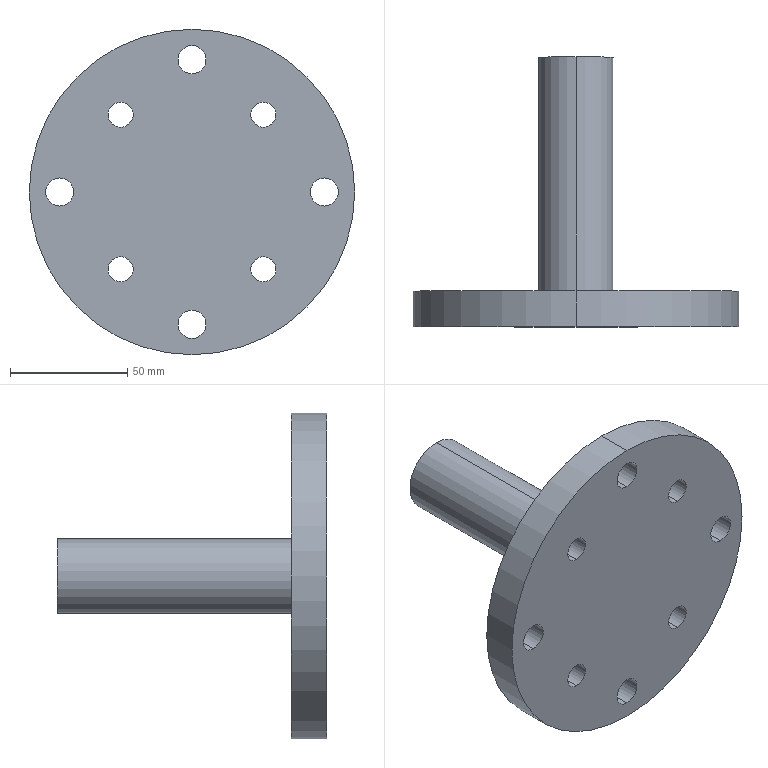Part | SolidWorks | features ICE 4, Cut 1, Extrusion 1, Scale 1 | 1 solid | 26 faces | box 139 x 115.24 x 139 mm | volume 246251 mm3 | cylinder 22 | plane 4 | commonest cylinder face diameters 10.668 x8 12 x8 26 x2 32 x2 139 x2
STEP:
#1=CARTESIAN_POINT('',(0.,0.,-69.5));
#2=VERTEX_POINT('',#1);
#3=CARTESIAN_POINT('',(0.,0.,69.5));
#4=VERTEX_POINT('',#3);
#5=CARTESIAN_POINT('',(0.,0.,0.));
#6=DIRECTION('',(0.,-1.,0.));
#7=DIRECTION('',(0.,0.,1.));
#8=AXIS2_PLACEMENT_3D('',#5,#6,#7);
#9=CIRCLE('',#8,69.5);
#10=EDGE_CURVE('',#2,#4,#9,.T.);
#11=ORIENTED_EDGE('',*,*,#10,.T.);
#12=CARTESIAN_POINT('',(0.,-15.24,69.5));
#13=VERTEX_POINT('',#12);
#14=CARTESIAN_POINT('',(0.,196.576,69.5));
#15=DIRECTION('',(0.,-1.,0.));
#16=VECTOR('',#15,1000.);
#17=LINE('',#14,#16);
#18=EDGE_CURVE('',#4,#13,#17,.T.);
#19=ORIENTED_EDGE('',*,*,#18,.T.);
#20=CARTESIAN_POINT('',(0.,-15.24,-69.5));
#21=VERTEX_POINT('',#20);
#22=CARTESIAN_POINT('',(0.,-15.24,0.));
#23=DIRECTION('',(0.,-1.,0.));
#24=DIRECTION('',(0.,0.,-1.));
#25=AXIS2_PLACEMENT_3D('',#22,#23,#24);
#26=CIRCLE('',#25,69.5);
#27=EDGE_CURVE('',#21,#13,#26,.T.);
#28=ORIENTED_EDGE('',*,*,#27,.F.);
#29=CARTESIAN_POINT('',(0.,196.576,-69.5));
#30=DIRECTION('',(0.,-1.,0.));
#31=VECTOR('',#30,1000.);
#32=LINE('',#29,#31);
#33=EDGE_CURVE('',#2,#21,#32,.T.);
#34=ORIENTED_EDGE('',*,*,#33,.F.);
#35=EDGE_LOOP('',(#11,#19,#28,#34));
#36=FACE_OUTER_BOUND('',#35,.T.);
#37=CARTESIAN_POINT('',(0.,196.576,0.));
#38=DIRECTION('',(0.,-1.,0.));
#39=DIRECTION('',(0.,0.,-1.));
#40=AXIS2_PLACEMENT_3D('',#37,#38,#39);
#41=CYLINDRICAL_SURFACE('',#40,69.5);
#42=ADVANCED_FACE('',(#36),#41,.T.);
#43=CARTESIAN_POINT('',(56.569,-15.24,-6.));
#44=VERTEX_POINT('',#43);
#45=CARTESIAN_POINT('',(56.569,-15.24,6.));
#46=VERTEX_POINT('',#45);
#47=CARTESIAN_POINT('',(56.569,-15.24,0.));
#48=DIRECTION('',(0.,1.,0.));
#49=DIRECTION('',(0.,0.,1.));
#50=AXIS2_PLACEMENT_3D('',#47,#48,#49);
#51=CIRCLE('',#50,6.);
#52=EDGE_CURVE('',#44,#46,#51,.T.);
#53=ORIENTED_EDGE('',*,*,#52,.F.);
#54=CARTESIAN_POINT('',(56.569,0.,-6.));
#55=VERTEX_POINT('',#54);
#56=CARTESIAN_POINT('',(56.569,-21.,-6.));
#57=DIRECTION('',(0.,1.,0.));
#58=VECTOR('',#57,1000.);
#59=LINE('',#56,#58);
#60=EDGE_CURVE('',#44,#55,#59,.T.);
#61=ORIENTED_EDGE('',*,*,#60,.T.);
#62=CARTESIAN_POINT('',(56.569,0.,6.));
#63=VERTEX_POINT('',#62);
#64=CARTESIAN_POINT('',(56.569,0.,0.));
#65=DIRECTION('',(0.,1.,0.));
#66=DIRECTION('',(0.,0.,1.));
#67=AXIS2_PLACEMENT_3D('',#64,#65,#66);
#68=CIRCLE('',#67,6.);
#69=EDGE_CURVE('',#55,#63,#68,.T.);
#70=ORIENTED_EDGE('',*,*,#69,.T.);
#71=CARTESIAN_POINT('',(56.569,-21.,6.));
#72=DIRECTION('',(0.,1.,0.));
#73=VECTOR('',#72,1000.);
#74=LINE('',#71,#73);
#75=EDGE_CURVE('',#46,#63,#74,.T.);
#76=ORIENTED_EDGE('',*,*,#75,.F.);
#77=EDGE_LOOP('',(#53,#61,#70,#76));
#78=FACE_OUTER_BOUND('',#77,.T.);
#79=CARTESIAN_POINT('',(56.569,-21.,0.));
#80=DIRECTION('',(0.,1.,0.));
#81=DIRECTION('',(0.,0.,1.));
#82=AXIS2_PLACEMENT_3D('',#79,#80,#81);
#83=CYLINDRICAL_SURFACE('',#82,6.);
#84=ADVANCED_FACE('',(#78),#83,.F.);
#85=CARTESIAN_POINT('',(0.,-15.24,50.569));
#86=VERTEX_POINT('',#85);
#87=CARTESIAN_POINT('',(0.,-15.24,62.569));
#88=VERTEX_POINT('',#87);
#89=CARTESIAN_POINT('',(0.,-15.24,56.569));
#90=DIRECTION('',(0.,1.,0.));
#91=DIRECTION('',(0.,0.,1.));
#92=AXIS2_PLACEMENT_3D('',#89,#90,#91);
#93=CIRCLE('',#92,6.);
#94=EDGE_CURVE('',#86,#88,#93,.T.);
#95=ORIENTED_EDGE('',*,*,#94,.F.);
#96=CARTESIAN_POINT('',(0.,0.,50.569));
#97=VERTEX_POINT('',#96);
#98=CARTESIAN_POINT('',(0.,-21.,50.569));
#99=DIRECTION('',(0.,1.,0.));
#100=VECTOR('',#99,1000.);
#101=LINE('',#98,#100);
#102=EDGE_CURVE('',#86,#97,#101,.T.);
#103=ORIENTED_EDGE('',*,*,#102,.T.);
#104=CARTESIAN_POINT('',(0.,0.,62.569));
#105=VERTEX_POINT('',#104);
#106=CARTESIAN_POINT('',(0.,0.,56.569));
#107=DIRECTION('',(0.,1.,0.));
#108=DIRECTION('',(0.,0.,1.));
#109=AXIS2_PLACEMENT_3D('',#106,#107,#108);
#110=CIRCLE('',#109,6.);
#111=EDGE_CURVE('',#97,#105,#110,.T.);
#112=ORIENTED_EDGE('',*,*,#111,.T.);
#113=CARTESIAN_POINT('',(0.,-21.,62.569));
#114=DIRECTION('',(0.,1.,0.));
#115=VECTOR('',#114,1000.);
#116=LINE('',#113,#115);
#117=EDGE_CURVE('',#88,#105,#116,.T.);
#118=ORIENTED_EDGE('',*,*,#117,.F.);
#119=EDGE_LOOP('',(#95,#103,#112,#118));
#120=FACE_OUTER_BOUND('',#119,.T.);
#121=CARTESIAN_POINT('',(0.,-21.,56.569));
#122=DIRECTION('',(0.,1.,0.));
#123=DIRECTION('',(0.,0.,1.));
#124=AXIS2_PLACEMENT_3D('',#121,#122,#123);
#125=CYLINDRICAL_SURFACE('',#124,6.);
#126=ADVANCED_FACE('',(#120),#125,.F.);
#127=CARTESIAN_POINT('',(-56.569,-15.24,-6.));
#128=VERTEX_POINT('',#127);
#129=CARTESIAN_POINT('',(-56.569,-15.24,6.));
#130=VERTEX_POINT('',#129);
#131=CARTESIAN_POINT('',(-56.569,-15.24,0.));
#132=DIRECTION('',(0.,1.,0.));
#133=DIRECTION('',(0.,0.,1.));
#134=AXIS2_PLACEMENT_3D('',#131,#132,#133);
#135=CIRCLE('',#134,6.);
#136=EDGE_CURVE('',#128,#130,#135,.T.);
#137=ORIENTED_EDGE('',*,*,#136,.F.);
#138=CARTESIAN_POINT('',(-56.569,0.,-6.));
#139=VERTEX_POINT('',#138);
#140=CARTESIAN_POINT('',(-56.569,-21.,-6.));
#141=DIRECTION('',(0.,1.,0.));
#142=VECTOR('',#141,1000.);
#143=LINE('',#140,#142);
#144=EDGE_CURVE('',#128,#139,#143,.T.);
#145=ORIENTED_EDGE('',*,*,#144,.T.);
#146=CARTESIAN_POINT('',(-56.569,0.,6.));
#147=VERTEX_POINT('',#146);
#148=CARTESIAN_POINT('',(-56.569,0.,0.));
#149=DIRECTION('',(0.,1.,0.));
#150=DIRECTION('',(0.,0.,1.));
#151=AXIS2_PLACEMENT_3D('',#148,#149,#150);
#152=CIRCLE('',#151,6.);
#153=EDGE_CURVE('',#139,#147,#152,.T.);
#154=ORIENTED_EDGE('',*,*,#153,.T.);
#155=CARTESIAN_POINT('',(-56.569,-21.,6.));
#156=DIRECTION('',(0.,1.,0.));
#157=VECTOR('',#156,1000.);
#158=LINE('',#155,#157);
#159=EDGE_CURVE('',#130,#147,#158,.T.);
#160=ORIENTED_EDGE('',*,*,#159,.F.);
#161=EDGE_LOOP('',(#137,#145,#154,#160));
#162=FACE_OUTER_BOUND('',#161,.T.);
#163=CARTESIAN_POINT('',(-56.569,-21.,0.));
#164=DIRECTION('',(0.,1.,0.));
#165=DIRECTION('',(0.,0.,1.));
#166=AXIS2_PLACEMENT_3D('',#163,#164,#165);
#167=CYLINDRICAL_SURFACE('',#166,6.);
#168=ADVANCED_FACE('',(#162),#167,.F.);
#169=CARTESIAN_POINT('',(0.,-15.24,-62.569));
#170=VERTEX_POINT('',#169);
#171=CARTESIAN_POINT('',(0.,-15.24,-50.569));
#172=VERTEX_POINT('',#171);
#173=CARTESIAN_POINT('',(0.,-15.24,-56.569));
#174=DIRECTION('',(0.,1.,0.));
#175=DIRECTION('',(0.,0.,1.));
#176=AXIS2_PLACEMENT_3D('',#173,#174,#175);
#177=CIRCLE('',#176,6.);
#178=EDGE_CURVE('',#170,#172,#177,.T.);
#179=ORIENTED_EDGE('',*,*,#178,.F.);
#180=CARTESIAN_POINT('',(0.,0.,-62.569));
#181=VERTEX_POINT('',#180);
#182=CARTESIAN_POINT('',(0.,-21.,-62.569));
#183=DIRECTION('',(0.,1.,0.));
#184=VECTOR('',#183,1000.);
#185=LINE('',#182,#184);
#186=EDGE_CURVE('',#170,#181,#185,.T.);
#187=ORIENTED_EDGE('',*,*,#186,.T.);
#188=CARTESIAN_POINT('',(0.,0.,-50.569));
#189=VERTEX_POINT('',#188);
#190=CARTESIAN_POINT('',(0.,0.,-56.569));
#191=DIRECTION('',(0.,1.,0.));
#192=DIRECTION('',(0.,0.,1.));
#193=AXIS2_PLACEMENT_3D('',#190,#191,#192);
#194=CIRCLE('',#193,6.);
#195=EDGE_CURVE('',#181,#189,#194,.T.);
#196=ORIENTED_EDGE('',*,*,#195,.T.);
#197=CARTESIAN_POINT('',(0.,-21.,-50.569));
#198=DIRECTION('',(0.,1.,0.));
#199=VECTOR('',#198,1000.);
#200=LINE('',#197,#199);
#201=EDGE_CURVE('',#172,#189,#200,.T.);
#202=ORIENTED_EDGE('',*,*,#201,.F.);
#203=EDGE_LOOP('',(#179,#187,#196,#202));
#204=FACE_OUTER_BOUND('',#203,.T.);
#205=CARTESIAN_POINT('',(0.,-21.,-56.569));
#206=DIRECTION('',(0.,1.,0.));
#207=DIRECTION('',(0.,0.,1.));
#208=AXIS2_PLACEMENT_3D('',#205,#206,#207);
#209=CYLINDRICAL_SURFACE('',#208,6.);
#210=ADVANCED_FACE('',(#204),#209,.F.);
#211=CARTESIAN_POINT('',(0.,100.,-13.));
#212=VERTEX_POINT('',#211);
#213=CARTESIAN_POINT('',(0.,100.,13.));
#214=VERTEX_POINT('',#213);
#215=CARTESIAN_POINT('',(0.,100.,0.));
#216=DIRECTION('',(0.,1.,0.));
#217=DIRECTION('',(0.,0.,1.));
#218=AXIS2_PLACEMENT_3D('',#215,#216,#217);
#219=CIRCLE('',#218,13.);
#220=EDGE_CURVE('',#212,#214,#219,.T.);
#221=ORIENTED_EDGE('',*,*,#220,.T.);
#222=CARTESIAN_POINT('',(0.,0.,13.));
#223=VERTEX_POINT('',#222);
#224=CARTESIAN_POINT('',(0.,100.,13.));
#225=DIRECTION('',(0.,-1.,0.));
#226=VECTOR('',#225,1000.);
#227=LINE('',#224,#226);
#228=EDGE_CURVE('',#214,#223,#227,.T.);
#229=ORIENTED_EDGE('',*,*,#228,.T.);
#230=CARTESIAN_POINT('',(0.,0.,-13.));
#231=VERTEX_POINT('',#230);
#232=CARTESIAN_POINT('',(0.,0.,0.));
#233=DIRECTION('',(0.,-1.,0.));
#234=DIRECTION('',(0.,0.,1.));
#235=AXIS2_PLACEMENT_3D('',#232,#233,#234);
#236=CIRCLE('',#235,13.);
#237=EDGE_CURVE('',#223,#231,#236,.T.);
#238=ORIENTED_EDGE('',*,*,#237,.T.);
#239=CARTESIAN_POINT('',(0.,100.,-13.));
#240=DIRECTION('',(0.,-1.,0.));
#241=VECTOR('',#240,1000.);
#242=LINE('',#239,#241);
#243=EDGE_CURVE('',#212,#231,#242,.T.);
#244=ORIENTED_EDGE('',*,*,#243,.F.);
#245=EDGE_LOOP('',(#221,#229,#238,#244));
#246=FACE_OUTER_BOUND('',#245,.T.);
#247=CARTESIAN_POINT('',(0.,100.,0.));
#248=DIRECTION('',(0.,-1.,0.));
#249=DIRECTION('',(0.,0.,-1.));
#250=AXIS2_PLACEMENT_3D('',#247,#248,#249);
#251=CYLINDRICAL_SURFACE('',#250,13.);
#252=ADVANCED_FACE('',(#246),#251,.F.);
#253=CARTESIAN_POINT('',(0.,100.,16.));
#254=VERTEX_POINT('',#253);
#255=CARTESIAN_POINT('',(0.,100.,-16.));
#256=VERTEX_POINT('',#255);
#257=CARTESIAN_POINT('',(0.,100.,0.));
#258=DIRECTION('',(0.,1.,0.));
#259=DIRECTION('',(0.,0.,1.));
#260=AXIS2_PLACEMENT_3D('',#257,#258,#259);
#261=CIRCLE('',#260,16.);
#262=EDGE_CURVE('',#254,#256,#261,.T.);
#263=ORIENTED_EDGE('',*,*,#262,.F.);
#264=CARTESIAN_POINT('',(0.,0.,16.));
#265=VERTEX_POINT('',#264);
#266=CARTESIAN_POINT('',(0.,100.,16.));
#267=DIRECTION('',(0.,-1.,0.));
#268=VECTOR('',#267,1000.);
#269=LINE('',#266,#268);
#270=EDGE_CURVE('',#254,#265,#269,.T.);
#271=ORIENTED_EDGE('',*,*,#270,.T.);
#272=CARTESIAN_POINT('',(0.,0.,-16.));
#273=VERTEX_POINT('',#272);
#274=CARTESIAN_POINT('',(0.,0.,0.));
#275=DIRECTION('',(0.,1.,0.));
#276=DIRECTION('',(0.,0.,1.));
#277=AXIS2_PLACEMENT_3D('',#274,#275,#276);
#278=CIRCLE('',#277,16.);
#279=EDGE_CURVE('',#265,#273,#278,.T.);
#280=ORIENTED_EDGE('',*,*,#279,.T.);
#281=CARTESIAN_POINT('',(0.,100.,-16.));
#282=DIRECTION('',(0.,-1.,0.));
#283=VECTOR('',#282,1000.);
#284=LINE('',#281,#283);
#285=EDGE_CURVE('',#256,#273,#284,.T.);
#286=ORIENTED_EDGE('',*,*,#285,.F.);
#287=EDGE_LOOP('',(#263,#271,#280,#286));
#288=FACE_OUTER_BOUND('',#287,.T.);
#289=CARTESIAN_POINT('',(0.,100.,0.));
#290=DIRECTION('',(0.,-1.,0.));
#291=DIRECTION('',(0.,0.,-1.));
#292=AXIS2_PLACEMENT_3D('',#289,#290,#291);
#293=CYLINDRICAL_SURFACE('',#292,16.);
#294=ADVANCED_FACE('',(#288),#293,.T.);
#295=CARTESIAN_POINT('',(-30.48,-15.24,27.686));
#296=VERTEX_POINT('',#295);
#297=CARTESIAN_POINT('',(-30.48,-15.24,38.354));
#298=VERTEX_POINT('',#297);
#299=CARTESIAN_POINT('',(-30.48,-15.24,33.02));
#300=DIRECTION('',(0.,1.,0.));
#301=DIRECTION('',(0.,0.,1.));
#302=AXIS2_PLACEMENT_3D('',#299,#300,#301);
#303=CIRCLE('',#302,5.334);
#304=EDGE_CURVE('',#296,#298,#303,.T.);
#305=ORIENTED_EDGE('',*,*,#304,.F.);
#306=CARTESIAN_POINT('',(-30.48,0.,27.686));
#307=VERTEX_POINT('',#306);
#308=CARTESIAN_POINT('',(-30.48,-15.24,27.686));
#309=DIRECTION('',(0.,1.,0.));
#310=VECTOR('',#309,1000.);
#311=LINE('',#308,#310);
#312=EDGE_CURVE('',#296,#307,#311,.T.);
#313=ORIENTED_EDGE('',*,*,#312,.T.);
#314=CARTESIAN_POINT('',(-30.48,0.,38.354));
#315=VERTEX_POINT('',#314);
#316=CARTESIAN_POINT('',(-30.48,0.,33.02));
#317=DIRECTION('',(0.,1.,0.));
#318=DIRECTION('',(0.,0.,1.));
#319=AXIS2_PLACEMENT_3D('',#316,#317,#318);
#320=CIRCLE('',#319,5.334);
#321=EDGE_CURVE('',#307,#315,#320,.T.);
#322=ORIENTED_EDGE('',*,*,#321,.T.);
#323=CARTESIAN_POINT('',(-30.48,-15.24,38.354));
#324=DIRECTION('',(0.,1.,0.));
#325=VECTOR('',#324,1000.);
#326=LINE('',#323,#325);
#327=EDGE_CURVE('',#298,#315,#326,.T.);
#328=ORIENTED_EDGE('',*,*,#327,.F.);
#329=EDGE_LOOP('',(#305,#313,#322,#328));
#330=FACE_OUTER_BOUND('',#329,.T.);
#331=CARTESIAN_POINT('',(-30.48,-15.24,33.02));
#332=DIRECTION('',(0.,1.,0.));
#333=DIRECTION('',(0.,0.,1.));
#334=AXIS2_PLACEMENT_3D('',#331,#332,#333);
#335=CYLINDRICAL_SURFACE('',#334,5.334);
#336=ADVANCED_FACE('',(#330),#335,.F.);
#337=CARTESIAN_POINT('',(30.48,-15.24,27.686));
#338=VERTEX_POINT('',#337);
#339=CARTESIAN_POINT('',(30.48,-15.24,38.354));
#340=VERTEX_POINT('',#339);
#341=CARTESIAN_POINT('',(30.48,-15.24,33.02));
#342=DIRECTION('',(0.,1.,0.));
#343=DIRECTION('',(0.,0.,1.));
#344=AXIS2_PLACEMENT_3D('',#341,#342,#343);
#345=CIRCLE('',#344,5.334);
#346=EDGE_CURVE('',#338,#340,#345,.T.);
#347=ORIENTED_EDGE('',*,*,#346,.F.);
#348=CARTESIAN_POINT('',(30.48,0.,27.686));
#349=VERTEX_POINT('',#348);
#350=CARTESIAN_POINT('',(30.48,-15.24,27.686));
#351=DIRECTION('',(0.,1.,0.));
#352=VECTOR('',#351,1000.);
#353=LINE('',#350,#352);
#354=EDGE_CURVE('',#338,#349,#353,.T.);
#355=ORIENTED_EDGE('',*,*,#354,.T.);
#356=CARTESIAN_POINT('',(30.48,0.,38.354));
#357=VERTEX_POINT('',#356);
#358=CARTESIAN_POINT('',(30.48,0.,33.02));
#359=DIRECTION('',(0.,1.,0.));
#360=DIRECTION('',(0.,0.,1.));
#361=AXIS2_PLACEMENT_3D('',#358,#359,#360);
#362=CIRCLE('',#361,5.334);
#363=EDGE_CURVE('',#349,#357,#362,.T.);
#364=ORIENTED_EDGE('',*,*,#363,.T.);
#365=CARTESIAN_POINT('',(30.48,-15.24,38.354));
#366=DIRECTION('',(0.,1.,0.));
#367=VECTOR('',#366,1000.);
#368=LINE('',#365,#367);
#369=EDGE_CURVE('',#340,#357,#368,.T.);
#370=ORIENTED_EDGE('',*,*,#369,.F.);
#371=EDGE_LOOP('',(#347,#355,#364,#370));
#372=FACE_OUTER_BOUND('',#371,.T.);
#373=CARTESIAN_POINT('',(30.48,-15.24,33.02));
#374=DIRECTION('',(0.,1.,0.));
#375=DIRECTION('',(0.,0.,1.));
#376=AXIS2_PLACEMENT_3D('',#373,#374,#375);
#377=CYLINDRICAL_SURFACE('',#376,5.334);
#378=ADVANCED_FACE('',(#372),#377,.F.);
#379=CARTESIAN_POINT('',(30.48,-15.24,-38.354));
#380=VERTEX_POINT('',#379);
#381=CARTESIAN_POINT('',(30.48,-15.24,-27.686));
#382=VERTEX_POINT('',#381);
#383=CARTESIAN_POINT('',(30.48,-15.24,-33.02));
#384=DIRECTION('',(0.,1.,0.));
#385=DIRECTION('',(0.,0.,1.));
#386=AXIS2_PLACEMENT_3D('',#383,#384,#385);
#387=CIRCLE('',#386,5.334);
#388=EDGE_CURVE('',#380,#382,#387,.T.);
#389=ORIENTED_EDGE('',*,*,#388,.F.);
#390=CARTESIAN_POINT('',(30.48,0.,-38.354));
#391=VERTEX_POINT('',#390);
#392=CARTESIAN_POINT('',(30.48,-15.24,-38.354));
#393=DIRECTION('',(0.,1.,0.));
#394=VECTOR('',#393,1000.);
#395=LINE('',#392,#394);
#396=EDGE_CURVE('',#380,#391,#395,.T.);
#397=ORIENTED_EDGE('',*,*,#396,.T.);
#398=CARTESIAN_POINT('',(30.48,0.,-27.686));
#399=VERTEX_POINT('',#398);
#400=CARTESIAN_POINT('',(30.48,0.,-33.02));
#401=DIRECTION('',(0.,1.,0.));
#402=DIRECTION('',(0.,0.,1.));
#403=AXIS2_PLACEMENT_3D('',#400,#401,#402);
#404=CIRCLE('',#403,5.334);
#405=EDGE_CURVE('',#391,#399,#404,.T.);
#406=ORIENTED_EDGE('',*,*,#405,.T.);
#407=CARTESIAN_POINT('',(30.48,-15.24,-27.686));
#408=DIRECTION('',(0.,1.,0.));
#409=VECTOR('',#408,1000.);
#410=LINE('',#407,#409);
#411=EDGE_CURVE('',#382,#399,#410,.T.);
#412=ORIENTED_EDGE('',*,*,#411,.F.);
#413=EDGE_LOOP('',(#389,#397,#406,#412));
#414=FACE_OUTER_BOUND('',#413,.T.);
#415=CARTESIAN_POINT('',(30.48,-15.24,-33.02));
#416=DIRECTION('',(0.,1.,0.));
#417=DIRECTION('',(0.,0.,1.));
#418=AXIS2_PLACEMENT_3D('',#415,#416,#417);
#419=CYLINDRICAL_SURFACE('',#418,5.334);
#420=ADVANCED_FACE('',(#414),#419,.F.);
#421=CARTESIAN_POINT('',(-30.48,-15.24,-38.354));
#422=VERTEX_POINT('',#421);
#423=CARTESIAN_POINT('',(-30.48,-15.24,-27.686));
#424=VERTEX_POINT('',#423);
#425=CARTESIAN_POINT('',(-30.48,-15.24,-33.02));
#426=DIRECTION('',(0.,1.,0.));
#427=DIRECTION('',(0.,0.,1.));
#428=AXIS2_PLACEMENT_3D('',#425,#426,#427);
#429=CIRCLE('',#428,5.334);
#430=EDGE_CURVE('',#422,#424,#429,.T.);
#431=ORIENTED_EDGE('',*,*,#430,.F.);
#432=CARTESIAN_POINT('',(-30.48,0.,-38.354));
#433=VERTEX_POINT('',#432);
#434=CARTESIAN_POINT('',(-30.48,-15.24,-38.354));
#435=DIRECTION('',(0.,1.,0.));
#436=VECTOR('',#435,1000.);
#437=LINE('',#434,#436);
#438=EDGE_CURVE('',#422,#433,#437,.T.);
#439=ORIENTED_EDGE('',*,*,#438,.T.);
#440=CARTESIAN_POINT('',(-30.48,0.,-27.686));
#441=VERTEX_POINT('',#440);
#442=CARTESIAN_POINT('',(-30.48,0.,-33.02));
#443=DIRECTION('',(0.,1.,0.));
#444=DIRECTION('',(0.,0.,1.));
#445=AXIS2_PLACEMENT_3D('',#442,#443,#444);
#446=CIRCLE('',#445,5.334);
#447=EDGE_CURVE('',#433,#441,#446,.T.);
#448=ORIENTED_EDGE('',*,*,#447,.T.);
#449=CARTESIAN_POINT('',(-30.48,-15.24,-27.686));
#450=DIRECTION('',(0.,1.,0.));
#451=VECTOR('',#450,1000.);
#452=LINE('',#449,#451);
#453=EDGE_CURVE('',#424,#441,#452,.T.);
#454=ORIENTED_EDGE('',*,*,#453,.F.);
#455=EDGE_LOOP('',(#431,#439,#448,#454));
#456=FACE_OUTER_BOUND('',#455,.T.);
#457=CARTESIAN_POINT('',(-30.48,-15.24,-33.02));
#458=DIRECTION('',(0.,1.,0.));
#459=DIRECTION('',(0.,0.,1.));
#460=AXIS2_PLACEMENT_3D('',#457,#458,#459);
#461=CYLINDRICAL_SURFACE('',#460,5.334);
#462=ADVANCED_FACE('',(#456),#461,.F.);
#463=CARTESIAN_POINT('',(56.569,-15.24,0.));
#464=DIRECTION('',(0.,1.,0.));
#465=DIRECTION('',(0.,0.,1.));
#466=AXIS2_PLACEMENT_3D('',#463,#464,#465);
#467=CIRCLE('',#466,6.);
#468=EDGE_CURVE('',#46,#44,#467,.T.);
#469=ORIENTED_EDGE('',*,*,#468,.T.);
#470=ORIENTED_EDGE('',*,*,#52,.T.);
#471=EDGE_LOOP('',(#469,#470));
#472=FACE_BOUND('',#471,.T.);
#473=CARTESIAN_POINT('',(0.,-15.24,56.569));
#474=DIRECTION('',(0.,1.,0.));
#475=DIRECTION('',(0.,0.,1.));
#476=AXIS2_PLACEMENT_3D('',#473,#474,#475);
#477=CIRCLE('',#476,6.);
#478=EDGE_CURVE('',#88,#86,#477,.T.);
#479=ORIENTED_EDGE('',*,*,#478,.T.);
#480=ORIENTED_EDGE('',*,*,#94,.T.);
#481=EDGE_LOOP('',(#479,#480));
#482=FACE_BOUND('',#481,.T.);
#483=CARTESIAN_POINT('',(-56.569,-15.24,0.));
#484=DIRECTION('',(0.,1.,0.));
#485=DIRECTION('',(0.,0.,1.));
#486=AXIS2_PLACEMENT_3D('',#483,#484,#485);
#487=CIRCLE('',#486,6.);
#488=EDGE_CURVE('',#130,#128,#487,.T.);
#489=ORIENTED_EDGE('',*,*,#488,.T.);
#490=ORIENTED_EDGE('',*,*,#136,.T.);
#491=EDGE_LOOP('',(#489,#490));
#492=FACE_BOUND('',#491,.T.);
#493=CARTESIAN_POINT('',(0.,-15.24,-56.569));
#494=DIRECTION('',(0.,1.,0.));
#495=DIRECTION('',(0.,0.,1.));
#496=AXIS2_PLACEMENT_3D('',#493,#494,#495);
#497=CIRCLE('',#496,6.);
#498=EDGE_CURVE('',#172,#170,#497,.T.);
#499=ORIENTED_EDGE('',*,*,#498,.T.);
#500=ORIENTED_EDGE('',*,*,#178,.T.);
#501=EDGE_LOOP('',(#499,#500));
#502=FACE_BOUND('',#501,.T.);
#503=CARTESIAN_POINT('',(-30.48,-15.24,33.02));
#504=DIRECTION('',(0.,1.,0.));
#505=DIRECTION('',(0.,0.,1.));
#506=AXIS2_PLACEMENT_3D('',#503,#504,#505);
#507=CIRCLE('',#506,5.334);
#508=EDGE_CURVE('',#298,#296,#507,.T.);
#509=ORIENTED_EDGE('',*,*,#508,.T.);
#510=ORIENTED_EDGE('',*,*,#304,.T.);
#511=EDGE_LOOP('',(#509,#510));
#512=FACE_BOUND('',#511,.T.);
#513=CARTESIAN_POINT('',(30.48,-15.24,33.02));
#514=DIRECTION('',(0.,1.,0.));
#515=DIRECTION('',(0.,0.,1.));
#516=AXIS2_PLACEMENT_3D('',#513,#514,#515);
#517=CIRCLE('',#516,5.334);
#518=EDGE_CURVE('',#340,#338,#517,.T.);
#519=ORIENTED_EDGE('',*,*,#518,.T.);
#520=ORIENTED_EDGE('',*,*,#346,.T.);
#521=EDGE_LOOP('',(#519,#520));
#522=FACE_BOUND('',#521,.T.);
#523=CARTESIAN_POINT('',(30.48,-15.24,-33.02));
#524=DIRECTION('',(0.,1.,0.));
#525=DIRECTION('',(0.,0.,1.));
#526=AXIS2_PLACEMENT_3D('',#523,#524,#525);
#527=CIRCLE('',#526,5.334);
#528=EDGE_CURVE('',#382,#380,#527,.T.);
#529=ORIENTED_EDGE('',*,*,#528,.T.);
#530=ORIENTED_EDGE('',*,*,#388,.T.);
#531=EDGE_LOOP('',(#529,#530));
#532=FACE_BOUND('',#531,.T.);
#533=CARTESIAN_POINT('',(-30.48,-15.24,-33.02));
#534=DIRECTION('',(0.,1.,0.));
#535=DIRECTION('',(0.,0.,1.));
#536=AXIS2_PLACEMENT_3D('',#533,#534,#535);
#537=CIRCLE('',#536,5.334);
#538=EDGE_CURVE('',#424,#422,#537,.T.);
#539=ORIENTED_EDGE('',*,*,#538,.T.);
#540=ORIENTED_EDGE('',*,*,#430,.T.);
#541=EDGE_LOOP('',(#539,#540));
#542=FACE_BOUND('',#541,.T.);
#543=ORIENTED_EDGE('',*,*,#27,.T.);
#544=CARTESIAN_POINT('',(0.,-15.24,0.));
#545=DIRECTION('',(0.,-1.,0.));
#546=DIRECTION('',(0.,0.,-1.));
#547=AXIS2_PLACEMENT_3D('',#544,#545,#546);
#548=CIRCLE('',#547,69.5);
#549=EDGE_CURVE('',#13,#21,#548,.T.);
#550=ORIENTED_EDGE('',*,*,#549,.T.);
#551=EDGE_LOOP('',(#543,#550));
#552=FACE_OUTER_BOUND('',#551,.T.);
#553=CARTESIAN_POINT('',(0.,-15.24,0.));
#554=DIRECTION('',(0.,1.,0.));
#555=DIRECTION('',(0.,0.,1.));
#556=AXIS2_PLACEMENT_3D('',#553,#554,#555);
#557=PLANE('',#556);
#558=ADVANCED_FACE('',(#472,#482,#492,#502,#512,#522,#532,#542,#552),#557,.F.);
#559=CARTESIAN_POINT('',(56.569,0.,0.));
#560=DIRECTION('',(0.,1.,0.));
#561=DIRECTION('',(0.,0.,1.));
#562=AXIS2_PLACEMENT_3D('',#559,#560,#561);
#563=CIRCLE('',#562,6.);
#564=EDGE_CURVE('',#63,#55,#563,.T.);
#565=ORIENTED_EDGE('',*,*,#564,.F.);
#566=ORIENTED_EDGE('',*,*,#69,.F.);
#567=EDGE_LOOP('',(#565,#566));
#568=FACE_BOUND('',#567,.T.);
#569=CARTESIAN_POINT('',(0.,0.,56.569));
#570=DIRECTION('',(0.,1.,0.));
#571=DIRECTION('',(0.,0.,1.));
#572=AXIS2_PLACEMENT_3D('',#569,#570,#571);
#573=CIRCLE('',#572,6.);
#574=EDGE_CURVE('',#105,#97,#573,.T.);
#575=ORIENTED_EDGE('',*,*,#574,.F.);
#576=ORIENTED_EDGE('',*,*,#111,.F.);
#577=EDGE_LOOP('',(#575,#576));
#578=FACE_BOUND('',#577,.T.);
#579=CARTESIAN_POINT('',(-56.569,0.,0.));
#580=DIRECTION('',(0.,1.,0.));
#581=DIRECTION('',(0.,0.,1.));
#582=AXIS2_PLACEMENT_3D('',#579,#580,#581);
#583=CIRCLE('',#582,6.);
#584=EDGE_CURVE('',#147,#139,#583,.T.);
#585=ORIENTED_EDGE('',*,*,#584,.F.);
#586=ORIENTED_EDGE('',*,*,#153,.F.);
#587=EDGE_LOOP('',(#585,#586));
#588=FACE_BOUND('',#587,.T.);
#589=CARTESIAN_POINT('',(0.,0.,-56.569));
#590=DIRECTION('',(0.,1.,0.));
#591=DIRECTION('',(0.,0.,1.));
#592=AXIS2_PLACEMENT_3D('',#589,#590,#591);
#593=CIRCLE('',#592,6.);
#594=EDGE_CURVE('',#189,#181,#593,.T.);
#595=ORIENTED_EDGE('',*,*,#594,.F.);
#596=ORIENTED_EDGE('',*,*,#195,.F.);
#597=EDGE_LOOP('',(#595,#596));
#598=FACE_BOUND('',#597,.T.);
#599=CARTESIAN_POINT('',(0.,0.,0.));
#600=DIRECTION('',(0.,1.,0.));
#601=DIRECTION('',(0.,0.,1.));
#602=AXIS2_PLACEMENT_3D('',#599,#600,#601);
#603=CIRCLE('',#602,16.);
#604=EDGE_CURVE('',#273,#265,#603,.T.);
#605=ORIENTED_EDGE('',*,*,#604,.F.);
#606=ORIENTED_EDGE('',*,*,#279,.F.);
#607=EDGE_LOOP('',(#605,#606));
#608=FACE_BOUND('',#607,.T.);
#609=CARTESIAN_POINT('',(-30.48,0.,33.02));
#610=DIRECTION('',(0.,1.,0.));
#611=DIRECTION('',(0.,0.,1.));
#612=AXIS2_PLACEMENT_3D('',#609,#610,#611);
#613=CIRCLE('',#612,5.334);
#614=EDGE_CURVE('',#315,#307,#613,.T.);
#615=ORIENTED_EDGE('',*,*,#614,.F.);
#616=ORIENTED_EDGE('',*,*,#321,.F.);
#617=EDGE_LOOP('',(#615,#616));
#618=FACE_BOUND('',#617,.T.);
#619=CARTESIAN_POINT('',(30.48,0.,33.02));
#620=DIRECTION('',(0.,1.,0.));
#621=DIRECTION('',(0.,0.,1.));
#622=AXIS2_PLACEMENT_3D('',#619,#620,#621);
#623=CIRCLE('',#622,5.334);
#624=EDGE_CURVE('',#357,#349,#623,.T.);
#625=ORIENTED_EDGE('',*,*,#624,.F.);
#626=ORIENTED_EDGE('',*,*,#363,.F.);
#627=EDGE_LOOP('',(#625,#626));
#628=FACE_BOUND('',#627,.T.);
#629=CARTESIAN_POINT('',(30.48,0.,-33.02));
#630=DIRECTION('',(0.,1.,0.));
#631=DIRECTION('',(0.,0.,1.));
#632=AXIS2_PLACEMENT_3D('',#629,#630,#631);
#633=CIRCLE('',#632,5.334);
#634=EDGE_CURVE('',#399,#391,#633,.T.);
#635=ORIENTED_EDGE('',*,*,#634,.F.);
#636=ORIENTED_EDGE('',*,*,#405,.F.);
#637=EDGE_LOOP('',(#635,#636));
#638=FACE_BOUND('',#637,.T.);
#639=CARTESIAN_POINT('',(-30.48,0.,-33.02));
#640=DIRECTION('',(0.,1.,0.));
#641=DIRECTION('',(0.,0.,1.));
#642=AXIS2_PLACEMENT_3D('',#639,#640,#641);
#643=CIRCLE('',#642,5.334);
#644=EDGE_CURVE('',#441,#433,#643,.T.);
#645=ORIENTED_EDGE('',*,*,#644,.F.);
#646=ORIENTED_EDGE('',*,*,#447,.F.);
#647=EDGE_LOOP('',(#645,#646));
#648=FACE_BOUND('',#647,.T.);
#649=ORIENTED_EDGE('',*,*,#10,.F.);
#650=CARTESIAN_POINT('',(0.,0.,0.));
#651=DIRECTION('',(0.,-1.,0.));
#652=DIRECTION('',(0.,0.,1.));
#653=AXIS2_PLACEMENT_3D('',#650,#651,#652);
#654=CIRCLE('',#653,69.5);
#655=EDGE_CURVE('',#4,#2,#654,.T.);
#656=ORIENTED_EDGE('',*,*,#655,.F.);
#657=EDGE_LOOP('',(#649,#656));
#658=FACE_OUTER_BOUND('',#657,.T.);
#659=CARTESIAN_POINT('',(0.,0.,0.));
#660=DIRECTION('',(0.,1.,0.));
#661=DIRECTION('',(0.,0.,1.));
#662=AXIS2_PLACEMENT_3D('',#659,#660,#661);
#663=PLANE('',#662);
#664=ADVANCED_FACE('',(#568,#578,#588,#598,#608,#618,#628,#638,#648,#658),#663,.T.);
#665=ORIENTED_EDGE('',*,*,#438,.F.);
#666=ORIENTED_EDGE('',*,*,#538,.F.);
#667=ORIENTED_EDGE('',*,*,#453,.T.);
#668=ORIENTED_EDGE('',*,*,#644,.T.);
#669=EDGE_LOOP('',(#665,#666,#667,#668));
#670=FACE_OUTER_BOUND('',#669,.T.);
#671=CARTESIAN_POINT('',(-30.48,-15.24,-33.02));
#672=DIRECTION('',(0.,1.,0.));
#673=DIRECTION('',(0.,0.,1.));
#674=AXIS2_PLACEMENT_3D('',#671,#672,#673);
#675=CYLINDRICAL_SURFACE('',#674,5.334);
#676=ADVANCED_FACE('',(#670),#675,.F.);
#677=ORIENTED_EDGE('',*,*,#396,.F.);
#678=ORIENTED_EDGE('',*,*,#528,.F.);
#679=ORIENTED_EDGE('',*,*,#411,.T.);
#680=ORIENTED_EDGE('',*,*,#634,.T.);
#681=EDGE_LOOP('',(#677,#678,#679,#680));
#682=FACE_OUTER_BOUND('',#681,.T.);
#683=CARTESIAN_POINT('',(30.48,-15.24,-33.02));
#684=DIRECTION('',(0.,1.,0.));
#685=DIRECTION('',(0.,0.,1.));
#686=AXIS2_PLACEMENT_3D('',#683,#684,#685);
#687=CYLINDRICAL_SURFACE('',#686,5.334);
#688=ADVANCED_FACE('',(#682),#687,.F.);
#689=ORIENTED_EDGE('',*,*,#354,.F.);
#690=ORIENTED_EDGE('',*,*,#518,.F.);
#691=ORIENTED_EDGE('',*,*,#369,.T.);
#692=ORIENTED_EDGE('',*,*,#624,.T.);
#693=EDGE_LOOP('',(#689,#690,#691,#692));
#694=FACE_OUTER_BOUND('',#693,.T.);
#695=CARTESIAN_POINT('',(30.48,-15.24,33.02));
#696=DIRECTION('',(0.,1.,0.));
#697=DIRECTION('',(0.,0.,1.));
#698=AXIS2_PLACEMENT_3D('',#695,#696,#697);
#699=CYLINDRICAL_SURFACE('',#698,5.334);
#700=ADVANCED_FACE('',(#694),#699,.F.);
#701=ORIENTED_EDGE('',*,*,#312,.F.);
#702=ORIENTED_EDGE('',*,*,#508,.F.);
#703=ORIENTED_EDGE('',*,*,#327,.T.);
#704=ORIENTED_EDGE('',*,*,#614,.T.);
#705=EDGE_LOOP('',(#701,#702,#703,#704));
#706=FACE_OUTER_BOUND('',#705,.T.);
#707=CARTESIAN_POINT('',(-30.48,-15.24,33.02));
#708=DIRECTION('',(0.,1.,0.));
#709=DIRECTION('',(0.,0.,1.));
#710=AXIS2_PLACEMENT_3D('',#707,#708,#709);
#711=CYLINDRICAL_SURFACE('',#710,5.334);
#712=ADVANCED_FACE('',(#706),#711,.F.);
#713=CARTESIAN_POINT('',(0.,100.,0.));
#714=DIRECTION('',(0.,1.,0.));
#715=DIRECTION('',(0.,0.,1.));
#716=AXIS2_PLACEMENT_3D('',#713,#714,#715);
#717=CIRCLE('',#716,16.);
#718=EDGE_CURVE('',#256,#254,#717,.T.);
#719=ORIENTED_EDGE('',*,*,#718,.T.);
#720=ORIENTED_EDGE('',*,*,#262,.T.);
#721=EDGE_LOOP('',(#719,#720));
#722=FACE_OUTER_BOUND('',#721,.T.);
#723=ORIENTED_EDGE('',*,*,#220,.F.);
#724=CARTESIAN_POINT('',(0.,100.,0.));
#725=DIRECTION('',(0.,1.,0.));
#726=DIRECTION('',(0.,0.,1.));
#727=AXIS2_PLACEMENT_3D('',#724,#725,#726);
#728=CIRCLE('',#727,13.);
#729=EDGE_CURVE('',#214,#212,#728,.T.);
#730=ORIENTED_EDGE('',*,*,#729,.F.);
#731=EDGE_LOOP('',(#723,#730));
#732=FACE_BOUND('',#731,.T.);
#733=CARTESIAN_POINT('',(0.,100.,0.));
#734=DIRECTION('',(0.,1.,0.));
#735=DIRECTION('',(0.,0.,1.));
#736=AXIS2_PLACEMENT_3D('',#733,#734,#735);
#737=PLANE('',#736);
#738=ADVANCED_FACE('',(#722,#732),#737,.T.);
#739=ORIENTED_EDGE('',*,*,#270,.F.);
#740=ORIENTED_EDGE('',*,*,#718,.F.);
#741=ORIENTED_EDGE('',*,*,#285,.T.);
#742=ORIENTED_EDGE('',*,*,#604,.T.);
#743=EDGE_LOOP('',(#739,#740,#741,#742));
#744=FACE_OUTER_BOUND('',#743,.T.);
#745=CARTESIAN_POINT('',(0.,100.,0.));
#746=DIRECTION('',(0.,-1.,0.));
#747=DIRECTION('',(0.,0.,-1.));
#748=AXIS2_PLACEMENT_3D('',#745,#746,#747);
#749=CYLINDRICAL_SURFACE('',#748,16.);
#750=ADVANCED_FACE('',(#744),#749,.T.);
#751=ORIENTED_EDGE('',*,*,#228,.F.);
#752=ORIENTED_EDGE('',*,*,#729,.T.);
#753=ORIENTED_EDGE('',*,*,#243,.T.);
#754=CARTESIAN_POINT('',(0.,0.,0.));
#755=DIRECTION('',(0.,-1.,0.));
#756=DIRECTION('',(0.,0.,1.));
#757=AXIS2_PLACEMENT_3D('',#754,#755,#756);
#758=CIRCLE('',#757,13.);
#759=EDGE_CURVE('',#231,#223,#758,.T.);
#760=ORIENTED_EDGE('',*,*,#759,.T.);
#761=EDGE_LOOP('',(#751,#752,#753,#760));
#762=FACE_OUTER_BOUND('',#761,.T.);
#763=CARTESIAN_POINT('',(0.,100.,0.));
#764=DIRECTION('',(0.,-1.,0.));
#765=DIRECTION('',(0.,0.,-1.));
#766=AXIS2_PLACEMENT_3D('',#763,#764,#765);
#767=CYLINDRICAL_SURFACE('',#766,13.);
#768=ADVANCED_FACE('',(#762),#767,.F.);
#769=ORIENTED_EDGE('',*,*,#759,.F.);
#770=ORIENTED_EDGE('',*,*,#237,.F.);
#771=EDGE_LOOP('',(#769,#770));
#772=FACE_OUTER_BOUND('',#771,.T.);
#773=CARTESIAN_POINT('',(0.,0.,0.));
#774=DIRECTION('',(0.,1.,0.));
#775=DIRECTION('',(0.,0.,1.));
#776=AXIS2_PLACEMENT_3D('',#773,#774,#775);
#777=PLANE('',#776);
#778=ADVANCED_FACE('',(#772),#777,.T.);
#779=ORIENTED_EDGE('',*,*,#186,.F.);
#780=ORIENTED_EDGE('',*,*,#498,.F.);
#781=ORIENTED_EDGE('',*,*,#201,.T.);
#782=ORIENTED_EDGE('',*,*,#594,.T.);
#783=EDGE_LOOP('',(#779,#780,#781,#782));
#784=FACE_OUTER_BOUND('',#783,.T.);
#785=CARTESIAN_POINT('',(0.,-21.,-56.569));
#786=DIRECTION('',(0.,1.,0.));
#787=DIRECTION('',(0.,0.,1.));
#788=AXIS2_PLACEMENT_3D('',#785,#786,#787);
#789=CYLINDRICAL_SURFACE('',#788,6.);
#790=ADVANCED_FACE('',(#784),#789,.F.);
#791=ORIENTED_EDGE('',*,*,#144,.F.);
#792=ORIENTED_EDGE('',*,*,#488,.F.);
#793=ORIENTED_EDGE('',*,*,#159,.T.);
#794=ORIENTED_EDGE('',*,*,#584,.T.);
#795=EDGE_LOOP('',(#791,#792,#793,#794));
#796=FACE_OUTER_BOUND('',#795,.T.);
#797=CARTESIAN_POINT('',(-56.569,-21.,0.));
#798=DIRECTION('',(0.,1.,0.));
#799=DIRECTION('',(0.,0.,1.));
#800=AXIS2_PLACEMENT_3D('',#797,#798,#799);
#801=CYLINDRICAL_SURFACE('',#800,6.);
#802=ADVANCED_FACE('',(#796),#801,.F.);
#803=ORIENTED_EDGE('',*,*,#102,.F.);
#804=ORIENTED_EDGE('',*,*,#478,.F.);
#805=ORIENTED_EDGE('',*,*,#117,.T.);
#806=ORIENTED_EDGE('',*,*,#574,.T.);
#807=EDGE_LOOP('',(#803,#804,#805,#806));
#808=FACE_OUTER_BOUND('',#807,.T.);
#809=CARTESIAN_POINT('',(0.,-21.,56.569));
#810=DIRECTION('',(0.,1.,0.));
#811=DIRECTION('',(0.,0.,1.));
#812=AXIS2_PLACEMENT_3D('',#809,#810,#811);
#813=CYLINDRICAL_SURFACE('',#812,6.);
#814=ADVANCED_FACE('',(#808),#813,.F.);
#815=ORIENTED_EDGE('',*,*,#60,.F.);
#816=ORIENTED_EDGE('',*,*,#468,.F.);
#817=ORIENTED_EDGE('',*,*,#75,.T.);
#818=ORIENTED_EDGE('',*,*,#564,.T.);
#819=EDGE_LOOP('',(#815,#816,#817,#818));
#820=FACE_OUTER_BOUND('',#819,.T.);
#821=CARTESIAN_POINT('',(56.569,-21.,0.));
#822=DIRECTION('',(0.,1.,0.));
#823=DIRECTION('',(0.,0.,1.));
#824=AXIS2_PLACEMENT_3D('',#821,#822,#823);
#825=CYLINDRICAL_SURFACE('',#824,6.);
#826=ADVANCED_FACE('',(#820),#825,.F.);
#827=ORIENTED_EDGE('',*,*,#18,.F.);
#828=ORIENTED_EDGE('',*,*,#655,.T.);
#829=ORIENTED_EDGE('',*,*,#33,.T.);
#830=ORIENTED_EDGE('',*,*,#549,.F.);
#831=EDGE_LOOP('',(#827,#828,#829,#830));
#832=FACE_OUTER_BOUND('',#831,.T.);
#833=CARTESIAN_POINT('',(0.,196.576,0.));
#834=DIRECTION('',(0.,-1.,0.));
#835=DIRECTION('',(0.,0.,-1.));
#836=AXIS2_PLACEMENT_3D('',#833,#834,#835);
#837=CYLINDRICAL_SURFACE('',#836,69.5);
#838=ADVANCED_FACE('',(#832),#837,.T.);
#839=CLOSED_SHELL('',(#42,#84,#126,#168,#210,#252,#294,#336,#378,#420,#462,#558,#664,#676,#688,#700,#712,#738,#750,#768,#778,#790,#802,#814,#826,#838));
#840=MANIFOLD_SOLID_BREP('',#839);
#841=CARTESIAN_POINT('',(0.,0.,0.));
#842=DIRECTION('',(0.,0.,1.));
#843=DIRECTION('',(1.,0.,0.));
#844=AXIS2_PLACEMENT_3D('',#841,#842,#843);
#845=(LENGTH_UNIT()NAMED_UNIT(*)SI_UNIT(.MILLI.,.METRE.));
#846=UNCERTAINTY_MEASURE_WITH_UNIT(LENGTH_MEASURE(0.00001),#845,'','');
#847=(NAMED_UNIT(*)PLANE_ANGLE_UNIT()SI_UNIT($,.RADIAN.));
#848=(NAMED_UNIT(*)SI_UNIT($,.STERADIAN.)SOLID_ANGLE_UNIT());
#849=(GEOMETRIC_REPRESENTATION_CONTEXT(3)GLOBAL_UNCERTAINTY_ASSIGNED_CONTEXT((#846))GLOBAL_UNIT_ASSIGNED_CONTEXT((#845,#847,#848))REPRESENTATION_CONTEXT('',''));
#850=ADVANCED_BREP_SHAPE_REPRESENTATION('',(#840,#844),#849);